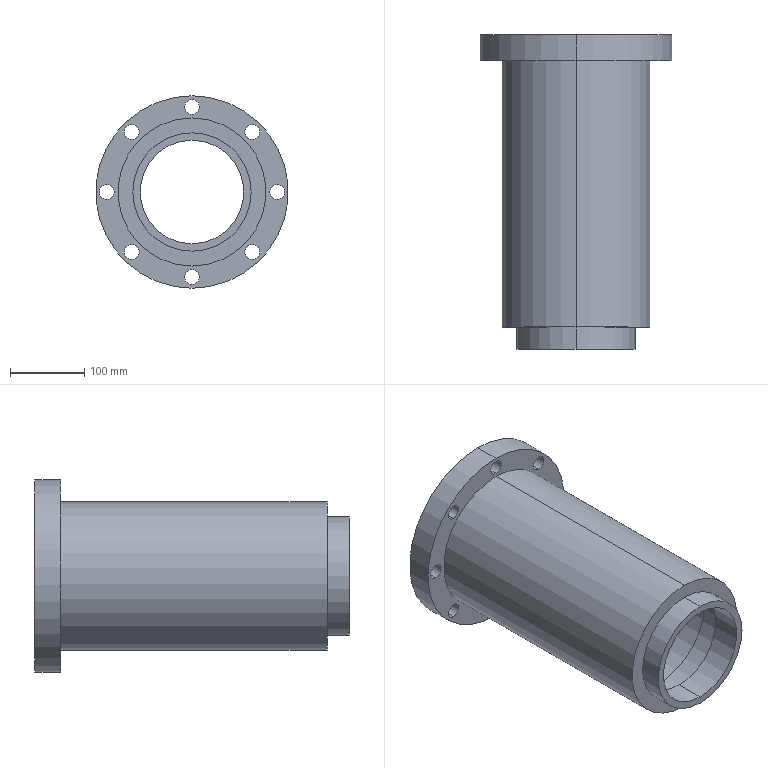Part | SolidWorks | features Cut 3, ICE 2, CirPattern 1, Extrusion 1, Shell 1 | 2 solids | 37 faces | box 260 x 425 x 260 mm | volume 2163536 mm3 | cylinder 30 | plane 7 | commonest cylinder face diameters 20 x16 200 x4 140 x2 160 x2 180 x2 190 x2
STEP:
#1=CARTESIAN_POINT('',(0.,51.,95.));
#2=VERTEX_POINT('',#1);
#3=CARTESIAN_POINT('',(0.,51.,-95.));
#4=VERTEX_POINT('',#3);
#5=CARTESIAN_POINT('',(0.,51.,0.));
#6=DIRECTION('',(0.,-1.,0.));
#7=DIRECTION('',(0.,0.,1.));
#8=AXIS2_PLACEMENT_3D('',#5,#6,#7);
#9=CIRCLE('',#8,95.);
#10=EDGE_CURVE('',#2,#4,#9,.T.);
#11=ORIENTED_EDGE('',*,*,#10,.T.);
#12=CARTESIAN_POINT('',(0.,360.,-95.));
#13=VERTEX_POINT('',#12);
#14=CARTESIAN_POINT('',(0.,-217.701,-95.));
#15=DIRECTION('',(0.,1.,0.));
#16=VECTOR('',#15,1000.);
#17=LINE('',#14,#16);
#18=EDGE_CURVE('',#4,#13,#17,.T.);
#19=ORIENTED_EDGE('',*,*,#18,.T.);
#20=CARTESIAN_POINT('',(0.,360.,95.));
#21=VERTEX_POINT('',#20);
#22=CARTESIAN_POINT('',(0.,360.,0.));
#23=DIRECTION('',(0.,1.,0.));
#24=DIRECTION('',(0.,0.,1.));
#25=AXIS2_PLACEMENT_3D('',#22,#23,#24);
#26=CIRCLE('',#25,95.);
#27=EDGE_CURVE('',#13,#21,#26,.T.);
#28=ORIENTED_EDGE('',*,*,#27,.T.);
#29=CARTESIAN_POINT('',(0.,-217.701,95.));
#30=DIRECTION('',(0.,1.,0.));
#31=VECTOR('',#30,1000.);
#32=LINE('',#29,#31);
#33=EDGE_CURVE('',#2,#21,#32,.T.);
#34=ORIENTED_EDGE('',*,*,#33,.F.);
#35=EDGE_LOOP('',(#11,#19,#28,#34));
#36=FACE_OUTER_BOUND('',#35,.T.);
#37=CARTESIAN_POINT('',(0.,-217.701,0.));
#38=DIRECTION('',(0.,1.,0.));
#39=DIRECTION('',(0.,0.,1.));
#40=AXIS2_PLACEMENT_3D('',#37,#38,#39);
#41=CYLINDRICAL_SURFACE('',#40,95.);
#42=ADVANCED_FACE('',(#36),#41,.F.);
#43=CARTESIAN_POINT('',(0.,-30.,-80.));
#44=VERTEX_POINT('',#43);
#45=CARTESIAN_POINT('',(0.,-30.,80.));
#46=VERTEX_POINT('',#45);
#47=CARTESIAN_POINT('',(0.,-30.,0.));
#48=DIRECTION('',(0.,-1.,0.));
#49=DIRECTION('',(0.,0.,-1.));
#50=AXIS2_PLACEMENT_3D('',#47,#48,#49);
#51=CIRCLE('',#50,80.);
#52=EDGE_CURVE('',#44,#46,#51,.T.);
#53=ORIENTED_EDGE('',*,*,#52,.F.);
#54=CARTESIAN_POINT('',(0.,0.,-80.));
#55=VERTEX_POINT('',#54);
#56=CARTESIAN_POINT('',(0.,-30.,-80.));
#57=DIRECTION('',(0.,1.,0.));
#58=VECTOR('',#57,1000.);
#59=LINE('',#56,#58);
#60=EDGE_CURVE('',#44,#55,#59,.T.);
#61=ORIENTED_EDGE('',*,*,#60,.T.);
#62=CARTESIAN_POINT('',(0.,0.,80.));
#63=VERTEX_POINT('',#62);
#64=CARTESIAN_POINT('',(0.,0.,0.));
#65=DIRECTION('',(0.,-1.,0.));
#66=DIRECTION('',(0.,0.,1.));
#67=AXIS2_PLACEMENT_3D('',#64,#65,#66);
#68=CIRCLE('',#67,80.);
#69=EDGE_CURVE('',#55,#63,#68,.T.);
#70=ORIENTED_EDGE('',*,*,#69,.T.);
#71=CARTESIAN_POINT('',(0.,-30.,80.));
#72=DIRECTION('',(0.,1.,0.));
#73=VECTOR('',#72,1000.);
#74=LINE('',#71,#73);
#75=EDGE_CURVE('',#46,#63,#74,.T.);
#76=ORIENTED_EDGE('',*,*,#75,.F.);
#77=EDGE_LOOP('',(#53,#61,#70,#76));
#78=FACE_OUTER_BOUND('',#77,.T.);
#79=CARTESIAN_POINT('',(0.,-30.,0.));
#80=DIRECTION('',(0.,1.,0.));
#81=DIRECTION('',(0.,0.,1.));
#82=AXIS2_PLACEMENT_3D('',#79,#80,#81);
#83=CYLINDRICAL_SURFACE('',#82,80.);
#84=ADVANCED_FACE('',(#78),#83,.T.);
#85=CARTESIAN_POINT('',(0.,-30.,70.));
#86=VERTEX_POINT('',#85);
#87=CARTESIAN_POINT('',(0.,-30.,-70.));
#88=VERTEX_POINT('',#87);
#89=CARTESIAN_POINT('',(0.,-30.,0.));
#90=DIRECTION('',(0.,-1.,0.));
#91=DIRECTION('',(0.,0.,-1.));
#92=AXIS2_PLACEMENT_3D('',#89,#90,#91);
#93=CIRCLE('',#92,70.);
#94=EDGE_CURVE('',#86,#88,#93,.T.);
#95=ORIENTED_EDGE('',*,*,#94,.T.);
#96=CARTESIAN_POINT('',(0.,10.,-70.));
#97=VERTEX_POINT('',#96);
#98=CARTESIAN_POINT('',(0.,-290.,-70.));
#99=DIRECTION('',(0.,1.,0.));
#100=VECTOR('',#99,1000.);
#101=LINE('',#98,#100);
#102=EDGE_CURVE('',#88,#97,#101,.T.);
#103=ORIENTED_EDGE('',*,*,#102,.T.);
#104=CARTESIAN_POINT('',(0.,10.,70.));
#105=VERTEX_POINT('',#104);
#106=CARTESIAN_POINT('',(0.,10.,0.));
#107=DIRECTION('',(0.,1.,0.));
#108=DIRECTION('',(0.,0.,1.));
#109=AXIS2_PLACEMENT_3D('',#106,#107,#108);
#110=CIRCLE('',#109,70.);
#111=EDGE_CURVE('',#97,#105,#110,.T.);
#112=ORIENTED_EDGE('',*,*,#111,.T.);
#113=CARTESIAN_POINT('',(0.,-290.,70.));
#114=DIRECTION('',(0.,1.,0.));
#115=VECTOR('',#114,1000.);
#116=LINE('',#113,#115);
#117=EDGE_CURVE('',#86,#105,#116,.T.);
#118=ORIENTED_EDGE('',*,*,#117,.F.);
#119=EDGE_LOOP('',(#95,#103,#112,#118));
#120=FACE_OUTER_BOUND('',#119,.T.);
#121=CARTESIAN_POINT('',(0.,-290.,0.));
#122=DIRECTION('',(0.,1.,0.));
#123=DIRECTION('',(0.,0.,1.));
#124=AXIS2_PLACEMENT_3D('',#121,#122,#123);
#125=CYLINDRICAL_SURFACE('',#124,70.);
#126=ADVANCED_FACE('',(#120),#125,.F.);
#127=CARTESIAN_POINT('',(0.,360.,100.));
#128=VERTEX_POINT('',#127);
#129=CARTESIAN_POINT('',(0.,360.,-100.));
#130=VERTEX_POINT('',#129);
#131=CARTESIAN_POINT('',(0.,360.,0.));
#132=DIRECTION('',(0.,1.,0.));
#133=DIRECTION('',(0.,0.,1.));
#134=AXIS2_PLACEMENT_3D('',#131,#132,#133);
#135=CIRCLE('',#134,100.);
#136=EDGE_CURVE('',#128,#130,#135,.T.);
#137=ORIENTED_EDGE('',*,*,#136,.F.);
#138=CARTESIAN_POINT('',(0.,0.,100.));
#139=VERTEX_POINT('',#138);
#140=CARTESIAN_POINT('',(0.,360.,100.));
#141=DIRECTION('',(0.,-1.,0.));
#142=VECTOR('',#141,1000.);
#143=LINE('',#140,#142);
#144=EDGE_CURVE('',#128,#139,#143,.T.);
#145=ORIENTED_EDGE('',*,*,#144,.T.);
#146=CARTESIAN_POINT('',(0.,0.,-100.));
#147=VERTEX_POINT('',#146);
#148=CARTESIAN_POINT('',(0.,0.,0.));
#149=DIRECTION('',(0.,1.,0.));
#150=DIRECTION('',(0.,0.,1.));
#151=AXIS2_PLACEMENT_3D('',#148,#149,#150);
#152=CIRCLE('',#151,100.);
#153=EDGE_CURVE('',#139,#147,#152,.T.);
#154=ORIENTED_EDGE('',*,*,#153,.T.);
#155=CARTESIAN_POINT('',(0.,360.,-100.));
#156=DIRECTION('',(0.,-1.,0.));
#157=VECTOR('',#156,1000.);
#158=LINE('',#155,#157);
#159=EDGE_CURVE('',#130,#147,#158,.T.);
#160=ORIENTED_EDGE('',*,*,#159,.F.);
#161=EDGE_LOOP('',(#137,#145,#154,#160));
#162=FACE_OUTER_BOUND('',#161,.T.);
#163=CARTESIAN_POINT('',(0.,360.,0.));
#164=DIRECTION('',(0.,-1.,0.));
#165=DIRECTION('',(0.,0.,-1.));
#166=AXIS2_PLACEMENT_3D('',#163,#164,#165);
#167=CYLINDRICAL_SURFACE('',#166,100.);
#168=ADVANCED_FACE('',(#162),#167,.T.);
#169=CARTESIAN_POINT('',(0.,51.,90.));
#170=VERTEX_POINT('',#169);
#171=CARTESIAN_POINT('',(0.,51.,-90.));
#172=VERTEX_POINT('',#171);
#173=CARTESIAN_POINT('',(0.,51.,0.));
#174=DIRECTION('',(0.,-1.,0.));
#175=DIRECTION('',(0.,0.,1.));
#176=AXIS2_PLACEMENT_3D('',#173,#174,#175);
#177=CIRCLE('',#176,90.);
#178=EDGE_CURVE('',#170,#172,#177,.T.);
#179=ORIENTED_EDGE('',*,*,#178,.F.);
#180=CARTESIAN_POINT('',(0.,10.,90.));
#181=VERTEX_POINT('',#180);
#182=CARTESIAN_POINT('',(0.,360.,90.));
#183=DIRECTION('',(0.,-1.,0.));
#184=VECTOR('',#183,1000.);
#185=LINE('',#182,#184);
#186=EDGE_CURVE('',#170,#181,#185,.T.);
#187=ORIENTED_EDGE('',*,*,#186,.T.);
#188=CARTESIAN_POINT('',(0.,10.,-90.));
#189=VERTEX_POINT('',#188);
#190=CARTESIAN_POINT('',(0.,10.,0.));
#191=DIRECTION('',(0.,1.,0.));
#192=DIRECTION('',(0.,0.,1.));
#193=AXIS2_PLACEMENT_3D('',#190,#191,#192);
#194=CIRCLE('',#193,90.);
#195=EDGE_CURVE('',#189,#181,#194,.T.);
#196=ORIENTED_EDGE('',*,*,#195,.F.);
#197=CARTESIAN_POINT('',(0.,360.,-90.));
#198=DIRECTION('',(0.,-1.,0.));
#199=VECTOR('',#198,1000.);
#200=LINE('',#197,#199);
#201=EDGE_CURVE('',#172,#189,#200,.T.);
#202=ORIENTED_EDGE('',*,*,#201,.F.);
#203=EDGE_LOOP('',(#179,#187,#196,#202));
#204=FACE_OUTER_BOUND('',#203,.T.);
#205=CARTESIAN_POINT('',(0.,360.,0.));
#206=DIRECTION('',(0.,-1.,0.));
#207=DIRECTION('',(0.,0.,-1.));
#208=AXIS2_PLACEMENT_3D('',#205,#206,#207);
#209=CYLINDRICAL_SURFACE('',#208,90.);
#210=ADVANCED_FACE('',(#204),#209,.F.);
#211=ORIENTED_EDGE('',*,*,#186,.F.);
#212=CARTESIAN_POINT('',(0.,51.,0.));
#213=DIRECTION('',(0.,-1.,0.));
#214=DIRECTION('',(0.,0.,1.));
#215=AXIS2_PLACEMENT_3D('',#212,#213,#214);
#216=CIRCLE('',#215,90.);
#217=EDGE_CURVE('',#172,#170,#216,.T.);
#218=ORIENTED_EDGE('',*,*,#217,.F.);
#219=ORIENTED_EDGE('',*,*,#201,.T.);
#220=CARTESIAN_POINT('',(0.,10.,0.));
#221=DIRECTION('',(0.,1.,0.));
#222=DIRECTION('',(0.,0.,1.));
#223=AXIS2_PLACEMENT_3D('',#220,#221,#222);
#224=CIRCLE('',#223,90.);
#225=EDGE_CURVE('',#181,#189,#224,.T.);
#226=ORIENTED_EDGE('',*,*,#225,.F.);
#227=EDGE_LOOP('',(#211,#218,#219,#226));
#228=FACE_OUTER_BOUND('',#227,.T.);
#229=CARTESIAN_POINT('',(0.,360.,0.));
#230=DIRECTION('',(0.,-1.,0.));
#231=DIRECTION('',(0.,0.,-1.));
#232=AXIS2_PLACEMENT_3D('',#229,#230,#231);
#233=CYLINDRICAL_SURFACE('',#232,90.);
#234=ADVANCED_FACE('',(#228),#233,.F.);
#235=CARTESIAN_POINT('',(0.,0.,0.));
#236=DIRECTION('',(0.,1.,0.));
#237=DIRECTION('',(0.,0.,1.));
#238=AXIS2_PLACEMENT_3D('',#235,#236,#237);
#239=CIRCLE('',#238,100.);
#240=EDGE_CURVE('',#147,#139,#239,.T.);
#241=ORIENTED_EDGE('',*,*,#240,.F.);
#242=ORIENTED_EDGE('',*,*,#153,.F.);
#243=EDGE_LOOP('',(#241,#242));
#244=FACE_OUTER_BOUND('',#243,.T.);
#245=CARTESIAN_POINT('',(0.,0.,0.));
#246=DIRECTION('',(0.,-1.,0.));
#247=DIRECTION('',(0.,0.,1.));
#248=AXIS2_PLACEMENT_3D('',#245,#246,#247);
#249=CIRCLE('',#248,80.);
#250=EDGE_CURVE('',#63,#55,#249,.T.);
#251=ORIENTED_EDGE('',*,*,#250,.F.);
#252=ORIENTED_EDGE('',*,*,#69,.F.);
#253=EDGE_LOOP('',(#251,#252));
#254=FACE_BOUND('',#253,.T.);
#255=CARTESIAN_POINT('',(0.,0.,0.));
#256=DIRECTION('',(0.,1.,0.));
#257=DIRECTION('',(0.,0.,1.));
#258=AXIS2_PLACEMENT_3D('',#255,#256,#257);
#259=PLANE('',#258);
#260=ADVANCED_FACE('',(#244,#254),#259,.F.);
#261=ORIENTED_EDGE('',*,*,#144,.F.);
#262=CARTESIAN_POINT('',(0.,360.,0.));
#263=DIRECTION('',(0.,1.,0.));
#264=DIRECTION('',(0.,0.,1.));
#265=AXIS2_PLACEMENT_3D('',#262,#263,#264);
#266=CIRCLE('',#265,100.);
#267=EDGE_CURVE('',#130,#128,#266,.T.);
#268=ORIENTED_EDGE('',*,*,#267,.F.);
#269=ORIENTED_EDGE('',*,*,#159,.T.);
#270=ORIENTED_EDGE('',*,*,#240,.T.);
#271=EDGE_LOOP('',(#261,#268,#269,#270));
#272=FACE_OUTER_BOUND('',#271,.T.);
#273=CARTESIAN_POINT('',(0.,360.,0.));
#274=DIRECTION('',(0.,-1.,0.));
#275=DIRECTION('',(0.,0.,-1.));
#276=AXIS2_PLACEMENT_3D('',#273,#274,#275);
#277=CYLINDRICAL_SURFACE('',#276,100.);
#278=ADVANCED_FACE('',(#272),#277,.T.);
#279=CARTESIAN_POINT('',(0.,360.,0.));
#280=DIRECTION('',(0.,1.,0.));
#281=DIRECTION('',(0.,0.,1.));
#282=AXIS2_PLACEMENT_3D('',#279,#280,#281);
#283=CIRCLE('',#282,95.);
#284=EDGE_CURVE('',#21,#13,#283,.T.);
#285=ORIENTED_EDGE('',*,*,#284,.F.);
#286=ORIENTED_EDGE('',*,*,#27,.F.);
#287=EDGE_LOOP('',(#285,#286));
#288=FACE_BOUND('',#287,.T.);
#289=ORIENTED_EDGE('',*,*,#267,.T.);
#290=ORIENTED_EDGE('',*,*,#136,.T.);
#291=EDGE_LOOP('',(#289,#290));
#292=FACE_OUTER_BOUND('',#291,.T.);
#293=CARTESIAN_POINT('',(0.,360.,0.));
#294=DIRECTION('',(0.,1.,0.));
#295=DIRECTION('',(0.,0.,1.));
#296=AXIS2_PLACEMENT_3D('',#293,#294,#295);
#297=PLANE('',#296);
#298=ADVANCED_FACE('',(#288,#292),#297,.T.);
#299=CARTESIAN_POINT('',(0.,10.,0.));
#300=DIRECTION('',(0.,1.,0.));
#301=DIRECTION('',(0.,0.,1.));
#302=AXIS2_PLACEMENT_3D('',#299,#300,#301);
#303=CIRCLE('',#302,70.);
#304=EDGE_CURVE('',#105,#97,#303,.T.);
#305=ORIENTED_EDGE('',*,*,#304,.F.);
#306=ORIENTED_EDGE('',*,*,#111,.F.);
#307=EDGE_LOOP('',(#305,#306));
#308=FACE_BOUND('',#307,.T.);
#309=ORIENTED_EDGE('',*,*,#195,.T.);
#310=ORIENTED_EDGE('',*,*,#225,.T.);
#311=EDGE_LOOP('',(#309,#310));
#312=FACE_OUTER_BOUND('',#311,.T.);
#313=CARTESIAN_POINT('',(0.,10.,0.));
#314=DIRECTION('',(0.,1.,0.));
#315=DIRECTION('',(0.,0.,1.));
#316=AXIS2_PLACEMENT_3D('',#313,#314,#315);
#317=PLANE('',#316);
#318=ADVANCED_FACE('',(#308,#312),#317,.T.);
#319=ORIENTED_EDGE('',*,*,#102,.F.);
#320=CARTESIAN_POINT('',(0.,-30.,0.));
#321=DIRECTION('',(0.,-1.,0.));
#322=DIRECTION('',(0.,0.,-1.));
#323=AXIS2_PLACEMENT_3D('',#320,#321,#322);
#324=CIRCLE('',#323,70.);
#325=EDGE_CURVE('',#88,#86,#324,.T.);
#326=ORIENTED_EDGE('',*,*,#325,.T.);
#327=ORIENTED_EDGE('',*,*,#117,.T.);
#328=ORIENTED_EDGE('',*,*,#304,.T.);
#329=EDGE_LOOP('',(#319,#326,#327,#328));
#330=FACE_OUTER_BOUND('',#329,.T.);
#331=CARTESIAN_POINT('',(0.,-290.,0.));
#332=DIRECTION('',(0.,1.,0.));
#333=DIRECTION('',(0.,0.,1.));
#334=AXIS2_PLACEMENT_3D('',#331,#332,#333);
#335=CYLINDRICAL_SURFACE('',#334,70.);
#336=ADVANCED_FACE('',(#330),#335,.F.);
#337=CARTESIAN_POINT('',(0.,-30.,0.));
#338=DIRECTION('',(0.,-1.,0.));
#339=DIRECTION('',(0.,0.,-1.));
#340=AXIS2_PLACEMENT_3D('',#337,#338,#339);
#341=CIRCLE('',#340,80.);
#342=EDGE_CURVE('',#46,#44,#341,.T.);
#343=ORIENTED_EDGE('',*,*,#342,.T.);
#344=ORIENTED_EDGE('',*,*,#52,.T.);
#345=EDGE_LOOP('',(#343,#344));
#346=FACE_OUTER_BOUND('',#345,.T.);
#347=ORIENTED_EDGE('',*,*,#94,.F.);
#348=ORIENTED_EDGE('',*,*,#325,.F.);
#349=EDGE_LOOP('',(#347,#348));
#350=FACE_BOUND('',#349,.T.);
#351=CARTESIAN_POINT('',(0.,-30.,0.));
#352=DIRECTION('',(0.,-1.,0.));
#353=DIRECTION('',(0.,0.,-1.));
#354=AXIS2_PLACEMENT_3D('',#351,#352,#353);
#355=PLANE('',#354);
#356=ADVANCED_FACE('',(#346,#350),#355,.T.);
#357=ORIENTED_EDGE('',*,*,#60,.F.);
#358=ORIENTED_EDGE('',*,*,#342,.F.);
#359=ORIENTED_EDGE('',*,*,#75,.T.);
#360=ORIENTED_EDGE('',*,*,#250,.T.);
#361=EDGE_LOOP('',(#357,#358,#359,#360));
#362=FACE_OUTER_BOUND('',#361,.T.);
#363=CARTESIAN_POINT('',(0.,-30.,0.));
#364=DIRECTION('',(0.,1.,0.));
#365=DIRECTION('',(0.,0.,1.));
#366=AXIS2_PLACEMENT_3D('',#363,#364,#365);
#367=CYLINDRICAL_SURFACE('',#366,80.);
#368=ADVANCED_FACE('',(#362),#367,.T.);
#369=ORIENTED_EDGE('',*,*,#18,.F.);
#370=CARTESIAN_POINT('',(0.,51.,0.));
#371=DIRECTION('',(0.,-1.,0.));
#372=DIRECTION('',(0.,0.,1.));
#373=AXIS2_PLACEMENT_3D('',#370,#371,#372);
#374=CIRCLE('',#373,95.);
#375=EDGE_CURVE('',#4,#2,#374,.T.);
#376=ORIENTED_EDGE('',*,*,#375,.T.);
#377=ORIENTED_EDGE('',*,*,#33,.T.);
#378=ORIENTED_EDGE('',*,*,#284,.T.);
#379=EDGE_LOOP('',(#369,#376,#377,#378));
#380=FACE_OUTER_BOUND('',#379,.T.);
#381=CARTESIAN_POINT('',(0.,-217.701,0.));
#382=DIRECTION('',(0.,1.,0.));
#383=DIRECTION('',(0.,0.,1.));
#384=AXIS2_PLACEMENT_3D('',#381,#382,#383);
#385=CYLINDRICAL_SURFACE('',#384,95.);
#386=ADVANCED_FACE('',(#380),#385,.F.);
#387=ORIENTED_EDGE('',*,*,#10,.F.);
#388=ORIENTED_EDGE('',*,*,#375,.F.);
#389=EDGE_LOOP('',(#387,#388));
#390=FACE_OUTER_BOUND('',#389,.T.);
#391=ORIENTED_EDGE('',*,*,#217,.T.);
#392=ORIENTED_EDGE('',*,*,#178,.T.);
#393=EDGE_LOOP('',(#391,#392));
#394=FACE_BOUND('',#393,.T.);
#395=CARTESIAN_POINT('',(0.,51.,0.));
#396=DIRECTION('',(0.,1.,0.));
#397=DIRECTION('',(-0.9024,0.,-0.4308));
#398=AXIS2_PLACEMENT_3D('',#395,#396,#397);
#399=PLANE('',#398);
#400=ADVANCED_FACE('',(#390,#394),#399,.T.);
#401=CLOSED_SHELL('',(#42,#84,#126,#168,#210,#234,#260,#278,#298,#318,#336,#356,#368,#386,#400));
#402=MANIFOLD_SOLID_BREP('',#401);
#403=CARTESIAN_POINT('',(0.,360.,105.));
#404=VERTEX_POINT('',#403);
#405=CARTESIAN_POINT('',(0.,360.,125.));
#406=VERTEX_POINT('',#405);
#407=CARTESIAN_POINT('',(0.,360.,115.));
#408=DIRECTION('',(0.,1.,0.));
#409=DIRECTION('',(1.,0.,0.));
#410=AXIS2_PLACEMENT_3D('',#407,#408,#409);
#411=CIRCLE('',#410,10.);
#412=EDGE_CURVE('',#404,#406,#411,.T.);
#413=ORIENTED_EDGE('',*,*,#412,.F.);
#414=CARTESIAN_POINT('',(0.,395.,105.));
#415=VERTEX_POINT('',#414);
#416=CARTESIAN_POINT('',(0.,360.,105.));
#417=DIRECTION('',(0.,1.,0.));
#418=VECTOR('',#417,1000.);
#419=LINE('',#416,#418);
#420=EDGE_CURVE('',#404,#415,#419,.T.);
#421=ORIENTED_EDGE('',*,*,#420,.T.);
#422=CARTESIAN_POINT('',(0.,395.,125.));
#423=VERTEX_POINT('',#422);
#424=CARTESIAN_POINT('',(0.,395.,115.));
#425=DIRECTION('',(0.,1.,0.));
#426=DIRECTION('',(0.,0.,1.));
#427=AXIS2_PLACEMENT_3D('',#424,#425,#426);
#428=CIRCLE('',#427,10.);
#429=EDGE_CURVE('',#415,#423,#428,.T.);
#430=ORIENTED_EDGE('',*,*,#429,.T.);
#431=CARTESIAN_POINT('',(0.,360.,125.));
#432=DIRECTION('',(0.,1.,0.));
#433=VECTOR('',#432,1000.);
#434=LINE('',#431,#433);
#435=EDGE_CURVE('',#406,#423,#434,.T.);
#436=ORIENTED_EDGE('',*,*,#435,.F.);
#437=EDGE_LOOP('',(#413,#421,#430,#436));
#438=FACE_OUTER_BOUND('',#437,.T.);
#439=CARTESIAN_POINT('',(0.,360.,115.));
#440=DIRECTION('',(0.,1.,0.));
#441=DIRECTION('',(0.,0.,1.));
#442=AXIS2_PLACEMENT_3D('',#439,#440,#441);
#443=CYLINDRICAL_SURFACE('',#442,10.);
#444=ADVANCED_FACE('',(#438),#443,.F.);
#445=CARTESIAN_POINT('',(81.317,360.,71.317));
#446=VERTEX_POINT('',#445);
#447=CARTESIAN_POINT('',(81.317,360.,91.317));
#448=VERTEX_POINT('',#447);
#449=CARTESIAN_POINT('',(81.317,360.,81.317));
#450=DIRECTION('',(0.,1.,0.));
#451=DIRECTION('',(0.7071,0.,-0.7071));
#452=AXIS2_PLACEMENT_3D('',#449,#450,#451);
#453=CIRCLE('',#452,10.);
#454=EDGE_CURVE('',#446,#448,#453,.T.);
#455=ORIENTED_EDGE('',*,*,#454,.F.);
#456=CARTESIAN_POINT('',(81.317,395.,71.317));
#457=VERTEX_POINT('',#456);
#458=CARTESIAN_POINT('',(81.317,360.,71.317));
#459=DIRECTION('',(0.,1.,0.));
#460=VECTOR('',#459,1000.);
#461=LINE('',#458,#460);
#462=EDGE_CURVE('',#446,#457,#461,.T.);
#463=ORIENTED_EDGE('',*,*,#462,.T.);
#464=CARTESIAN_POINT('',(81.317,395.,91.317));
#465=VERTEX_POINT('',#464);
#466=CARTESIAN_POINT('',(81.317,395.,81.317));
#467=DIRECTION('',(0.,1.,0.));
#468=DIRECTION('',(0.,0.,1.));
#469=AXIS2_PLACEMENT_3D('',#466,#467,#468);
#470=CIRCLE('',#469,10.);
#471=EDGE_CURVE('',#457,#465,#470,.T.);
#472=ORIENTED_EDGE('',*,*,#471,.T.);
#473=CARTESIAN_POINT('',(81.317,360.,91.317));
#474=DIRECTION('',(0.,1.,0.));
#475=VECTOR('',#474,1000.);
#476=LINE('',#473,#475);
#477=EDGE_CURVE('',#448,#465,#476,.T.);
#478=ORIENTED_EDGE('',*,*,#477,.F.);
#479=EDGE_LOOP('',(#455,#463,#472,#478));
#480=FACE_OUTER_BOUND('',#479,.T.);
#481=CARTESIAN_POINT('',(81.317,360.,81.317));
#482=DIRECTION('',(0.,1.,0.));
#483=DIRECTION('',(0.,0.,1.));
#484=AXIS2_PLACEMENT_3D('',#481,#482,#483);
#485=CYLINDRICAL_SURFACE('',#484,10.);
#486=ADVANCED_FACE('',(#480),#485,.F.);
#487=CARTESIAN_POINT('',(115.,360.,-10.));
#488=VERTEX_POINT('',#487);
#489=CARTESIAN_POINT('',(115.,360.,10.));
#490=VERTEX_POINT('',#489);
#491=CARTESIAN_POINT('',(115.,360.,0.));
#492=DIRECTION('',(0.,1.,0.));
#493=DIRECTION('',(0.,0.,-1.));
#494=AXIS2_PLACEMENT_3D('',#491,#492,#493);
#495=CIRCLE('',#494,10.);
#496=EDGE_CURVE('',#488,#490,#495,.T.);
#497=ORIENTED_EDGE('',*,*,#496,.F.);
#498=CARTESIAN_POINT('',(115.,395.,-10.));
#499=VERTEX_POINT('',#498);
#500=CARTESIAN_POINT('',(115.,360.,-10.));
#501=DIRECTION('',(0.,1.,0.));
#502=VECTOR('',#501,1000.);
#503=LINE('',#500,#502);
#504=EDGE_CURVE('',#488,#499,#503,.T.);
#505=ORIENTED_EDGE('',*,*,#504,.T.);
#506=CARTESIAN_POINT('',(115.,395.,10.));
#507=VERTEX_POINT('',#506);
#508=CARTESIAN_POINT('',(115.,395.,0.));
#509=DIRECTION('',(0.,1.,0.));
#510=DIRECTION('',(0.,0.,1.));
#511=AXIS2_PLACEMENT_3D('',#508,#509,#510);
#512=CIRCLE('',#511,10.);
#513=EDGE_CURVE('',#499,#507,#512,.T.);
#514=ORIENTED_EDGE('',*,*,#513,.T.);
#515=CARTESIAN_POINT('',(115.,360.,10.));
#516=DIRECTION('',(0.,1.,0.));
#517=VECTOR('',#516,1000.);
#518=LINE('',#515,#517);
#519=EDGE_CURVE('',#490,#507,#518,.T.);
#520=ORIENTED_EDGE('',*,*,#519,.F.);
#521=EDGE_LOOP('',(#497,#505,#514,#520));
#522=FACE_OUTER_BOUND('',#521,.T.);
#523=CARTESIAN_POINT('',(115.,360.,0.));
#524=DIRECTION('',(0.,1.,0.));
#525=DIRECTION('',(0.,0.,1.));
#526=AXIS2_PLACEMENT_3D('',#523,#524,#525);
#527=CYLINDRICAL_SURFACE('',#526,10.);
#528=ADVANCED_FACE('',(#522),#527,.F.);
#529=CARTESIAN_POINT('',(81.317,360.,-91.317));
#530=VERTEX_POINT('',#529);
#531=CARTESIAN_POINT('',(81.317,360.,-71.317));
#532=VERTEX_POINT('',#531);
#533=CARTESIAN_POINT('',(81.317,360.,-81.317));
#534=DIRECTION('',(0.,1.,0.));
#535=DIRECTION('',(-0.7071,0.,-0.7071));
#536=AXIS2_PLACEMENT_3D('',#533,#534,#535);
#537=CIRCLE('',#536,10.);
#538=EDGE_CURVE('',#530,#532,#537,.T.);
#539=ORIENTED_EDGE('',*,*,#538,.F.);
#540=CARTESIAN_POINT('',(81.317,395.,-91.317));
#541=VERTEX_POINT('',#540);
#542=CARTESIAN_POINT('',(81.317,360.,-91.317));
#543=DIRECTION('',(0.,1.,0.));
#544=VECTOR('',#543,1000.);
#545=LINE('',#542,#544);
#546=EDGE_CURVE('',#530,#541,#545,.T.);
#547=ORIENTED_EDGE('',*,*,#546,.T.);
#548=CARTESIAN_POINT('',(81.317,395.,-71.317));
#549=VERTEX_POINT('',#548);
#550=CARTESIAN_POINT('',(81.317,395.,-81.317));
#551=DIRECTION('',(0.,1.,0.));
#552=DIRECTION('',(0.,0.,1.));
#553=AXIS2_PLACEMENT_3D('',#550,#551,#552);
#554=CIRCLE('',#553,10.);
#555=EDGE_CURVE('',#541,#549,#554,.T.);
#556=ORIENTED_EDGE('',*,*,#555,.T.);
#557=CARTESIAN_POINT('',(81.317,360.,-71.317));
#558=DIRECTION('',(0.,1.,0.));
#559=VECTOR('',#558,1000.);
#560=LINE('',#557,#559);
#561=EDGE_CURVE('',#532,#549,#560,.T.);
#562=ORIENTED_EDGE('',*,*,#561,.F.);
#563=EDGE_LOOP('',(#539,#547,#556,#562));
#564=FACE_OUTER_BOUND('',#563,.T.);
#565=CARTESIAN_POINT('',(81.317,360.,-81.317));
#566=DIRECTION('',(0.,1.,0.));
#567=DIRECTION('',(0.,0.,1.));
#568=AXIS2_PLACEMENT_3D('',#565,#566,#567);
#569=CYLINDRICAL_SURFACE('',#568,10.);
#570=ADVANCED_FACE('',(#564),#569,.F.);
#571=CARTESIAN_POINT('',(0.,360.,-125.));
#572=VERTEX_POINT('',#571);
#573=CARTESIAN_POINT('',(0.,360.,-105.));
#574=VERTEX_POINT('',#573);
#575=CARTESIAN_POINT('',(0.,360.,-115.));
#576=DIRECTION('',(0.,1.,0.));
#577=DIRECTION('',(-1.,0.,0.));
#578=AXIS2_PLACEMENT_3D('',#575,#576,#577);
#579=CIRCLE('',#578,10.);
#580=EDGE_CURVE('',#572,#574,#579,.T.);
#581=ORIENTED_EDGE('',*,*,#580,.F.);
#582=CARTESIAN_POINT('',(0.,395.,-125.));
#583=VERTEX_POINT('',#582);
#584=CARTESIAN_POINT('',(0.,360.,-125.));
#585=DIRECTION('',(0.,1.,0.));
#586=VECTOR('',#585,1000.);
#587=LINE('',#584,#586);
#588=EDGE_CURVE('',#572,#583,#587,.T.);
#589=ORIENTED_EDGE('',*,*,#588,.T.);
#590=CARTESIAN_POINT('',(0.,395.,-105.));
#591=VERTEX_POINT('',#590);
#592=CARTESIAN_POINT('',(0.,395.,-115.));
#593=DIRECTION('',(0.,1.,0.));
#594=DIRECTION('',(0.,0.,1.));
#595=AXIS2_PLACEMENT_3D('',#592,#593,#594);
#596=CIRCLE('',#595,10.);
#597=EDGE_CURVE('',#583,#591,#596,.T.);
#598=ORIENTED_EDGE('',*,*,#597,.T.);
#599=CARTESIAN_POINT('',(0.,360.,-105.));
#600=DIRECTION('',(0.,1.,0.));
#601=VECTOR('',#600,1000.);
#602=LINE('',#599,#601);
#603=EDGE_CURVE('',#574,#591,#602,.T.);
#604=ORIENTED_EDGE('',*,*,#603,.F.);
#605=EDGE_LOOP('',(#581,#589,#598,#604));
#606=FACE_OUTER_BOUND('',#605,.T.);
#607=CARTESIAN_POINT('',(0.,360.,-115.));
#608=DIRECTION('',(0.,1.,0.));
#609=DIRECTION('',(0.,0.,1.));
#610=AXIS2_PLACEMENT_3D('',#607,#608,#609);
#611=CYLINDRICAL_SURFACE('',#610,10.);
#612=ADVANCED_FACE('',(#606),#611,.F.);
#613=CARTESIAN_POINT('',(-81.317,360.,-91.317));
#614=VERTEX_POINT('',#613);
#615=CARTESIAN_POINT('',(-81.317,360.,-71.317));
#616=VERTEX_POINT('',#615);
#617=CARTESIAN_POINT('',(-81.317,360.,-81.317));
#618=DIRECTION('',(0.,1.,0.));
#619=DIRECTION('',(-0.7071,0.,0.7071));
#620=AXIS2_PLACEMENT_3D('',#617,#618,#619);
#621=CIRCLE('',#620,10.);
#622=EDGE_CURVE('',#614,#616,#621,.T.);
#623=ORIENTED_EDGE('',*,*,#622,.F.);
#624=CARTESIAN_POINT('',(-81.317,395.,-91.317));
#625=VERTEX_POINT('',#624);
#626=CARTESIAN_POINT('',(-81.317,360.,-91.317));
#627=DIRECTION('',(0.,1.,0.));
#628=VECTOR('',#627,1000.);
#629=LINE('',#626,#628);
#630=EDGE_CURVE('',#614,#625,#629,.T.);
#631=ORIENTED_EDGE('',*,*,#630,.T.);
#632=CARTESIAN_POINT('',(-81.317,395.,-71.317));
#633=VERTEX_POINT('',#632);
#634=CARTESIAN_POINT('',(-81.317,395.,-81.317));
#635=DIRECTION('',(0.,1.,0.));
#636=DIRECTION('',(0.,0.,1.));
#637=AXIS2_PLACEMENT_3D('',#634,#635,#636);
#638=CIRCLE('',#637,10.);
#639=EDGE_CURVE('',#625,#633,#638,.T.);
#640=ORIENTED_EDGE('',*,*,#639,.T.);
#641=CARTESIAN_POINT('',(-81.317,360.,-71.317));
#642=DIRECTION('',(0.,1.,0.));
#643=VECTOR('',#642,1000.);
#644=LINE('',#641,#643);
#645=EDGE_CURVE('',#616,#633,#644,.T.);
#646=ORIENTED_EDGE('',*,*,#645,.F.);
#647=EDGE_LOOP('',(#623,#631,#640,#646));
#648=FACE_OUTER_BOUND('',#647,.T.);
#649=CARTESIAN_POINT('',(-81.317,360.,-81.317));
#650=DIRECTION('',(0.,1.,0.));
#651=DIRECTION('',(0.,0.,1.));
#652=AXIS2_PLACEMENT_3D('',#649,#650,#651);
#653=CYLINDRICAL_SURFACE('',#652,10.);
#654=ADVANCED_FACE('',(#648),#653,.F.);
#655=CARTESIAN_POINT('',(-81.317,360.,71.317));
#656=VERTEX_POINT('',#655);
#657=CARTESIAN_POINT('',(-81.317,360.,91.317));
#658=VERTEX_POINT('',#657);
#659=CARTESIAN_POINT('',(-81.317,360.,81.317));
#660=DIRECTION('',(0.,1.,0.));
#661=DIRECTION('',(0.7071,0.,0.7071));
#662=AXIS2_PLACEMENT_3D('',#659,#660,#661);
#663=CIRCLE('',#662,10.);
#664=EDGE_CURVE('',#656,#658,#663,.T.);
#665=ORIENTED_EDGE('',*,*,#664,.F.);
#666=CARTESIAN_POINT('',(-81.317,395.,71.317));
#667=VERTEX_POINT('',#666);
#668=CARTESIAN_POINT('',(-81.317,360.,71.317));
#669=DIRECTION('',(0.,1.,0.));
#670=VECTOR('',#669,1000.);
#671=LINE('',#668,#670);
#672=EDGE_CURVE('',#656,#667,#671,.T.);
#673=ORIENTED_EDGE('',*,*,#672,.T.);
#674=CARTESIAN_POINT('',(-81.317,395.,91.317));
#675=VERTEX_POINT('',#674);
#676=CARTESIAN_POINT('',(-81.317,395.,81.317));
#677=DIRECTION('',(0.,1.,0.));
#678=DIRECTION('',(0.,0.,1.));
#679=AXIS2_PLACEMENT_3D('',#676,#677,#678);
#680=CIRCLE('',#679,10.);
#681=EDGE_CURVE('',#667,#675,#680,.T.);
#682=ORIENTED_EDGE('',*,*,#681,.T.);
#683=CARTESIAN_POINT('',(-81.317,360.,91.317));
#684=DIRECTION('',(0.,1.,0.));
#685=VECTOR('',#684,1000.);
#686=LINE('',#683,#685);
#687=EDGE_CURVE('',#658,#675,#686,.T.);
#688=ORIENTED_EDGE('',*,*,#687,.F.);
#689=EDGE_LOOP('',(#665,#673,#682,#688));
#690=FACE_OUTER_BOUND('',#689,.T.);
#691=CARTESIAN_POINT('',(-81.317,360.,81.317));
#692=DIRECTION('',(0.,1.,0.));
#693=DIRECTION('',(0.,0.,1.));
#694=AXIS2_PLACEMENT_3D('',#691,#692,#693);
#695=CYLINDRICAL_SURFACE('',#694,10.);
#696=ADVANCED_FACE('',(#690),#695,.F.);
#697=CARTESIAN_POINT('',(-115.,360.,-10.));
#698=VERTEX_POINT('',#697);
#699=CARTESIAN_POINT('',(-115.,360.,10.));
#700=VERTEX_POINT('',#699);
#701=CARTESIAN_POINT('',(-115.,360.,0.));
#702=DIRECTION('',(0.,1.,0.));
#703=DIRECTION('',(0.,0.,1.));
#704=AXIS2_PLACEMENT_3D('',#701,#702,#703);
#705=CIRCLE('',#704,10.);
#706=EDGE_CURVE('',#698,#700,#705,.T.);
#707=ORIENTED_EDGE('',*,*,#706,.F.);
#708=CARTESIAN_POINT('',(-115.,395.,-10.));
#709=VERTEX_POINT('',#708);
#710=CARTESIAN_POINT('',(-115.,-30.,-10.));
#711=DIRECTION('',(0.,1.,0.));
#712=VECTOR('',#711,1000.);
#713=LINE('',#710,#712);
#714=EDGE_CURVE('',#698,#709,#713,.T.);
#715=ORIENTED_EDGE('',*,*,#714,.T.);
#716=CARTESIAN_POINT('',(-115.,395.,10.));
#717=VERTEX_POINT('',#716);
#718=CARTESIAN_POINT('',(-115.,395.,0.));
#719=DIRECTION('',(0.,1.,0.));
#720=DIRECTION('',(0.,0.,1.));
#721=AXIS2_PLACEMENT_3D('',#718,#719,#720);
#722=CIRCLE('',#721,10.);
#723=EDGE_CURVE('',#709,#717,#722,.T.);
#724=ORIENTED_EDGE('',*,*,#723,.T.);
#725=CARTESIAN_POINT('',(-115.,-30.,10.));
#726=DIRECTION('',(0.,1.,0.));
#727=VECTOR('',#726,1000.);
#728=LINE('',#725,#727);
#729=EDGE_CURVE('',#700,#717,#728,.T.);
#730=ORIENTED_EDGE('',*,*,#729,.F.);
#731=EDGE_LOOP('',(#707,#715,#724,#730));
#732=FACE_OUTER_BOUND('',#731,.T.);
#733=CARTESIAN_POINT('',(-115.,-30.,0.));
#734=DIRECTION('',(0.,1.,0.));
#735=DIRECTION('',(0.,0.,1.));
#736=AXIS2_PLACEMENT_3D('',#733,#734,#735);
#737=CYLINDRICAL_SURFACE('',#736,10.);
#738=ADVANCED_FACE('',(#732),#737,.F.);
#739=CARTESIAN_POINT('',(0.,395.,-100.));
#740=VERTEX_POINT('',#739);
#741=CARTESIAN_POINT('',(0.,395.,100.));
#742=VERTEX_POINT('',#741);
#743=CARTESIAN_POINT('',(0.,395.,0.));
#744=DIRECTION('',(0.,1.,0.));
#745=DIRECTION('',(0.,0.,1.));
#746=AXIS2_PLACEMENT_3D('',#743,#744,#745);
#747=CIRCLE('',#746,100.);
#748=EDGE_CURVE('',#740,#742,#747,.T.);
#749=ORIENTED_EDGE('',*,*,#748,.T.);
#750=CARTESIAN_POINT('',(0.,360.,100.));
#751=VERTEX_POINT('',#750);
#752=CARTESIAN_POINT('',(0.,395.,100.));
#753=DIRECTION('',(0.,-1.,0.));
#754=VECTOR('',#753,1000.);
#755=LINE('',#752,#754);
#756=EDGE_CURVE('',#742,#751,#755,.T.);
#757=ORIENTED_EDGE('',*,*,#756,.T.);
#758=CARTESIAN_POINT('',(0.,360.,-100.));
#759=VERTEX_POINT('',#758);
#760=CARTESIAN_POINT('',(0.,360.,0.));
#761=DIRECTION('',(0.,1.,0.));
#762=DIRECTION('',(0.,0.,1.));
#763=AXIS2_PLACEMENT_3D('',#760,#761,#762);
#764=CIRCLE('',#763,100.);
#765=EDGE_CURVE('',#759,#751,#764,.T.);
#766=ORIENTED_EDGE('',*,*,#765,.F.);
#767=CARTESIAN_POINT('',(0.,395.,-100.));
#768=DIRECTION('',(0.,-1.,0.));
#769=VECTOR('',#768,1000.);
#770=LINE('',#767,#769);
#771=EDGE_CURVE('',#740,#759,#770,.T.);
#772=ORIENTED_EDGE('',*,*,#771,.F.);
#773=EDGE_LOOP('',(#749,#757,#766,#772));
#774=FACE_OUTER_BOUND('',#773,.T.);
#775=CARTESIAN_POINT('',(0.,395.,0.));
#776=DIRECTION('',(0.,-1.,0.));
#777=DIRECTION('',(0.,0.,-1.));
#778=AXIS2_PLACEMENT_3D('',#775,#776,#777);
#779=CYLINDRICAL_SURFACE('',#778,100.);
#780=ADVANCED_FACE('',(#774),#779,.F.);
#781=CARTESIAN_POINT('',(0.,395.,130.));
#782=VERTEX_POINT('',#781);
#783=CARTESIAN_POINT('',(0.,395.,-130.));
#784=VERTEX_POINT('',#783);
#785=CARTESIAN_POINT('',(0.,395.,0.));
#786=DIRECTION('',(0.,1.,0.));
#787=DIRECTION('',(0.,0.,1.));
#788=AXIS2_PLACEMENT_3D('',#785,#786,#787);
#789=CIRCLE('',#788,130.);
#790=EDGE_CURVE('',#782,#784,#789,.T.);
#791=ORIENTED_EDGE('',*,*,#790,.F.);
#792=CARTESIAN_POINT('',(0.,360.,130.));
#793=VERTEX_POINT('',#792);
#794=CARTESIAN_POINT('',(0.,395.,130.));
#795=DIRECTION('',(0.,-1.,0.));
#796=VECTOR('',#795,1000.);
#797=LINE('',#794,#796);
#798=EDGE_CURVE('',#782,#793,#797,.T.);
#799=ORIENTED_EDGE('',*,*,#798,.T.);
#800=CARTESIAN_POINT('',(0.,360.,-130.));
#801=VERTEX_POINT('',#800);
#802=CARTESIAN_POINT('',(0.,360.,0.));
#803=DIRECTION('',(0.,1.,0.));
#804=DIRECTION('',(0.,0.,1.));
#805=AXIS2_PLACEMENT_3D('',#802,#803,#804);
#806=CIRCLE('',#805,130.);
#807=EDGE_CURVE('',#793,#801,#806,.T.);
#808=ORIENTED_EDGE('',*,*,#807,.T.);
#809=CARTESIAN_POINT('',(0.,395.,-130.));
#810=DIRECTION('',(0.,-1.,0.));
#811=VECTOR('',#810,1000.);
#812=LINE('',#809,#811);
#813=EDGE_CURVE('',#784,#801,#812,.T.);
#814=ORIENTED_EDGE('',*,*,#813,.F.);
#815=EDGE_LOOP('',(#791,#799,#808,#814));
#816=FACE_OUTER_BOUND('',#815,.T.);
#817=CARTESIAN_POINT('',(0.,395.,0.));
#818=DIRECTION('',(0.,-1.,0.));
#819=DIRECTION('',(0.,0.,-1.));
#820=AXIS2_PLACEMENT_3D('',#817,#818,#819);
#821=CYLINDRICAL_SURFACE('',#820,130.);
#822=ADVANCED_FACE('',(#816),#821,.T.);
#823=CARTESIAN_POINT('',(0.,395.,115.));
#824=DIRECTION('',(0.,1.,0.));
#825=DIRECTION('',(0.,0.,1.));
#826=AXIS2_PLACEMENT_3D('',#823,#824,#825);
#827=CIRCLE('',#826,10.);
#828=EDGE_CURVE('',#423,#415,#827,.T.);
#829=ORIENTED_EDGE('',*,*,#828,.F.);
#830=ORIENTED_EDGE('',*,*,#429,.F.);
#831=EDGE_LOOP('',(#829,#830));
#832=FACE_BOUND('',#831,.T.);
#833=CARTESIAN_POINT('',(81.317,395.,81.317));
#834=DIRECTION('',(0.,1.,0.));
#835=DIRECTION('',(0.,0.,1.));
#836=AXIS2_PLACEMENT_3D('',#833,#834,#835);
#837=CIRCLE('',#836,10.);
#838=EDGE_CURVE('',#465,#457,#837,.T.);
#839=ORIENTED_EDGE('',*,*,#838,.F.);
#840=ORIENTED_EDGE('',*,*,#471,.F.);
#841=EDGE_LOOP('',(#839,#840));
#842=FACE_BOUND('',#841,.T.);
#843=CARTESIAN_POINT('',(115.,395.,0.));
#844=DIRECTION('',(0.,1.,0.));
#845=DIRECTION('',(0.,0.,1.));
#846=AXIS2_PLACEMENT_3D('',#843,#844,#845);
#847=CIRCLE('',#846,10.);
#848=EDGE_CURVE('',#507,#499,#847,.T.);
#849=ORIENTED_EDGE('',*,*,#848,.F.);
#850=ORIENTED_EDGE('',*,*,#513,.F.);
#851=EDGE_LOOP('',(#849,#850));
#852=FACE_BOUND('',#851,.T.);
#853=CARTESIAN_POINT('',(81.317,395.,-81.317));
#854=DIRECTION('',(0.,1.,0.));
#855=DIRECTION('',(0.,0.,1.));
#856=AXIS2_PLACEMENT_3D('',#853,#854,#855);
#857=CIRCLE('',#856,10.);
#858=EDGE_CURVE('',#549,#541,#857,.T.);
#859=ORIENTED_EDGE('',*,*,#858,.F.);
#860=ORIENTED_EDGE('',*,*,#555,.F.);
#861=EDGE_LOOP('',(#859,#860));
#862=FACE_BOUND('',#861,.T.);
#863=CARTESIAN_POINT('',(0.,395.,-115.));
#864=DIRECTION('',(0.,1.,0.));
#865=DIRECTION('',(0.,0.,1.));
#866=AXIS2_PLACEMENT_3D('',#863,#864,#865);
#867=CIRCLE('',#866,10.);
#868=EDGE_CURVE('',#591,#583,#867,.T.);
#869=ORIENTED_EDGE('',*,*,#868,.F.);
#870=ORIENTED_EDGE('',*,*,#597,.F.);
#871=EDGE_LOOP('',(#869,#870));
#872=FACE_BOUND('',#871,.T.);
#873=CARTESIAN_POINT('',(-81.317,395.,-81.317));
#874=DIRECTION('',(0.,1.,0.));
#875=DIRECTION('',(0.,0.,1.));
#876=AXIS2_PLACEMENT_3D('',#873,#874,#875);
#877=CIRCLE('',#876,10.);
#878=EDGE_CURVE('',#633,#625,#877,.T.);
#879=ORIENTED_EDGE('',*,*,#878,.F.);
#880=ORIENTED_EDGE('',*,*,#639,.F.);
#881=EDGE_LOOP('',(#879,#880));
#882=FACE_BOUND('',#881,.T.);
#883=CARTESIAN_POINT('',(-81.317,395.,81.317));
#884=DIRECTION('',(0.,1.,0.));
#885=DIRECTION('',(0.,0.,1.));
#886=AXIS2_PLACEMENT_3D('',#883,#884,#885);
#887=CIRCLE('',#886,10.);
#888=EDGE_CURVE('',#675,#667,#887,.T.);
#889=ORIENTED_EDGE('',*,*,#888,.F.);
#890=ORIENTED_EDGE('',*,*,#681,.F.);
#891=EDGE_LOOP('',(#889,#890));
#892=FACE_BOUND('',#891,.T.);
#893=CARTESIAN_POINT('',(-115.,395.,0.));
#894=DIRECTION('',(0.,1.,0.));
#895=DIRECTION('',(0.,0.,1.));
#896=AXIS2_PLACEMENT_3D('',#893,#894,#895);
#897=CIRCLE('',#896,10.);
#898=EDGE_CURVE('',#717,#709,#897,.T.);
#899=ORIENTED_EDGE('',*,*,#898,.F.);
#900=ORIENTED_EDGE('',*,*,#723,.F.);
#901=EDGE_LOOP('',(#899,#900));
#902=FACE_BOUND('',#901,.T.);
#903=CARTESIAN_POINT('',(0.,395.,0.));
#904=DIRECTION('',(0.,1.,0.));
#905=DIRECTION('',(0.,0.,1.));
#906=AXIS2_PLACEMENT_3D('',#903,#904,#905);
#907=CIRCLE('',#906,130.);
#908=EDGE_CURVE('',#784,#782,#907,.T.);
#909=ORIENTED_EDGE('',*,*,#908,.T.);
#910=ORIENTED_EDGE('',*,*,#790,.T.);
#911=EDGE_LOOP('',(#909,#910));
#912=FACE_OUTER_BOUND('',#911,.T.);
#913=ORIENTED_EDGE('',*,*,#748,.F.);
#914=CARTESIAN_POINT('',(0.,395.,0.));
#915=DIRECTION('',(0.,1.,0.));
#916=DIRECTION('',(0.,0.,1.));
#917=AXIS2_PLACEMENT_3D('',#914,#915,#916);
#918=CIRCLE('',#917,100.);
#919=EDGE_CURVE('',#742,#740,#918,.T.);
#920=ORIENTED_EDGE('',*,*,#919,.F.);
#921=EDGE_LOOP('',(#913,#920));
#922=FACE_BOUND('',#921,.T.);
#923=CARTESIAN_POINT('',(0.,395.,0.));
#924=DIRECTION('',(0.,1.,0.));
#925=DIRECTION('',(0.,0.,1.));
#926=AXIS2_PLACEMENT_3D('',#923,#924,#925);
#927=PLANE('',#926);
#928=ADVANCED_FACE('',(#832,#842,#852,#862,#872,#882,#892,#902,#912,#922),#927,.T.);
#929=CARTESIAN_POINT('',(0.,360.,115.));
#930=DIRECTION('',(0.,1.,0.));
#931=DIRECTION('',(1.,0.,0.));
#932=AXIS2_PLACEMENT_3D('',#929,#930,#931);
#933=CIRCLE('',#932,10.);
#934=EDGE_CURVE('',#406,#404,#933,.T.);
#935=ORIENTED_EDGE('',*,*,#934,.T.);
#936=ORIENTED_EDGE('',*,*,#412,.T.);
#937=EDGE_LOOP('',(#935,#936));
#938=FACE_BOUND('',#937,.T.);
#939=CARTESIAN_POINT('',(81.317,360.,81.317));
#940=DIRECTION('',(0.,1.,0.));
#941=DIRECTION('',(0.7071,0.,-0.7071));
#942=AXIS2_PLACEMENT_3D('',#939,#940,#941);
#943=CIRCLE('',#942,10.);
#944=EDGE_CURVE('',#448,#446,#943,.T.);
#945=ORIENTED_EDGE('',*,*,#944,.T.);
#946=ORIENTED_EDGE('',*,*,#454,.T.);
#947=EDGE_LOOP('',(#945,#946));
#948=FACE_BOUND('',#947,.T.);
#949=CARTESIAN_POINT('',(115.,360.,0.));
#950=DIRECTION('',(0.,1.,0.));
#951=DIRECTION('',(0.,0.,-1.));
#952=AXIS2_PLACEMENT_3D('',#949,#950,#951);
#953=CIRCLE('',#952,10.);
#954=EDGE_CURVE('',#490,#488,#953,.T.);
#955=ORIENTED_EDGE('',*,*,#954,.T.);
#956=ORIENTED_EDGE('',*,*,#496,.T.);
#957=EDGE_LOOP('',(#955,#956));
#958=FACE_BOUND('',#957,.T.);
#959=CARTESIAN_POINT('',(81.317,360.,-81.317));
#960=DIRECTION('',(0.,1.,0.));
#961=DIRECTION('',(-0.7071,0.,-0.7071));
#962=AXIS2_PLACEMENT_3D('',#959,#960,#961);
#963=CIRCLE('',#962,10.);
#964=EDGE_CURVE('',#532,#530,#963,.T.);
#965=ORIENTED_EDGE('',*,*,#964,.T.);
#966=ORIENTED_EDGE('',*,*,#538,.T.);
#967=EDGE_LOOP('',(#965,#966));
#968=FACE_BOUND('',#967,.T.);
#969=CARTESIAN_POINT('',(0.,360.,-115.));
#970=DIRECTION('',(0.,1.,0.));
#971=DIRECTION('',(-1.,0.,0.));
#972=AXIS2_PLACEMENT_3D('',#969,#970,#971);
#973=CIRCLE('',#972,10.);
#974=EDGE_CURVE('',#574,#572,#973,.T.);
#975=ORIENTED_EDGE('',*,*,#974,.T.);
#976=ORIENTED_EDGE('',*,*,#580,.T.);
#977=EDGE_LOOP('',(#975,#976));
#978=FACE_BOUND('',#977,.T.);
#979=CARTESIAN_POINT('',(-81.317,360.,-81.317));
#980=DIRECTION('',(0.,1.,0.));
#981=DIRECTION('',(-0.7071,0.,0.7071));
#982=AXIS2_PLACEMENT_3D('',#979,#980,#981);
#983=CIRCLE('',#982,10.);
#984=EDGE_CURVE('',#616,#614,#983,.T.);
#985=ORIENTED_EDGE('',*,*,#984,.T.);
#986=ORIENTED_EDGE('',*,*,#622,.T.);
#987=EDGE_LOOP('',(#985,#986));
#988=FACE_BOUND('',#987,.T.);
#989=CARTESIAN_POINT('',(-81.317,360.,81.317));
#990=DIRECTION('',(0.,1.,0.));
#991=DIRECTION('',(0.7071,0.,0.7071));
#992=AXIS2_PLACEMENT_3D('',#989,#990,#991);
#993=CIRCLE('',#992,10.);
#994=EDGE_CURVE('',#658,#656,#993,.T.);
#995=ORIENTED_EDGE('',*,*,#994,.T.);
#996=ORIENTED_EDGE('',*,*,#664,.T.);
#997=EDGE_LOOP('',(#995,#996));
#998=FACE_BOUND('',#997,.T.);
#999=CARTESIAN_POINT('',(-115.,360.,0.));
#1000=DIRECTION('',(0.,1.,0.));
#1001=DIRECTION('',(0.,0.,1.));
#1002=AXIS2_PLACEMENT_3D('',#999,#1000,#1001);
#1003=CIRCLE('',#1002,10.);
#1004=EDGE_CURVE('',#700,#698,#1003,.T.);
#1005=ORIENTED_EDGE('',*,*,#1004,.T.);
#1006=ORIENTED_EDGE('',*,*,#706,.T.);
#1007=EDGE_LOOP('',(#1005,#1006));
#1008=FACE_BOUND('',#1007,.T.);
#1009=CARTESIAN_POINT('',(0.,360.,0.));
#1010=DIRECTION('',(0.,1.,0.));
#1011=DIRECTION('',(0.,0.,1.));
#1012=AXIS2_PLACEMENT_3D('',#1009,#1010,#1011);
#1013=CIRCLE('',#1012,130.);
#1014=EDGE_CURVE('',#801,#793,#1013,.T.);
#1015=ORIENTED_EDGE('',*,*,#1014,.F.);
#1016=ORIENTED_EDGE('',*,*,#807,.F.);
#1017=EDGE_LOOP('',(#1015,#1016));
#1018=FACE_OUTER_BOUND('',#1017,.T.);
#1019=ORIENTED_EDGE('',*,*,#765,.T.);
#1020=CARTESIAN_POINT('',(0.,360.,0.));
#1021=DIRECTION('',(0.,1.,0.));
#1022=DIRECTION('',(0.,0.,1.));
#1023=AXIS2_PLACEMENT_3D('',#1020,#1021,#1022);
#1024=CIRCLE('',#1023,100.);
#1025=EDGE_CURVE('',#751,#759,#1024,.T.);
#1026=ORIENTED_EDGE('',*,*,#1025,.T.);
#1027=EDGE_LOOP('',(#1019,#1026));
#1028=FACE_BOUND('',#1027,.T.);
#1029=CARTESIAN_POINT('',(0.,360.,0.));
#1030=DIRECTION('',(0.,1.,0.));
#1031=DIRECTION('',(0.,0.,1.));
#1032=AXIS2_PLACEMENT_3D('',#1029,#1030,#1031);
#1033=PLANE('',#1032);
#1034=ADVANCED_FACE('',(#938,#948,#958,#968,#978,#988,#998,#1008,#1018,#1028),#1033,.F.);
#1035=ORIENTED_EDGE('',*,*,#798,.F.);
#1036=ORIENTED_EDGE('',*,*,#908,.F.);
#1037=ORIENTED_EDGE('',*,*,#813,.T.);
#1038=ORIENTED_EDGE('',*,*,#1014,.T.);
#1039=EDGE_LOOP('',(#1035,#1036,#1037,#1038));
#1040=FACE_OUTER_BOUND('',#1039,.T.);
#1041=CARTESIAN_POINT('',(0.,395.,0.));
#1042=DIRECTION('',(0.,-1.,0.));
#1043=DIRECTION('',(0.,0.,-1.));
#1044=AXIS2_PLACEMENT_3D('',#1041,#1042,#1043);
#1045=CYLINDRICAL_SURFACE('',#1044,130.);
#1046=ADVANCED_FACE('',(#1040),#1045,.T.);
#1047=ORIENTED_EDGE('',*,*,#756,.F.);
#1048=ORIENTED_EDGE('',*,*,#919,.T.);
#1049=ORIENTED_EDGE('',*,*,#771,.T.);
#1050=ORIENTED_EDGE('',*,*,#1025,.F.);
#1051=EDGE_LOOP('',(#1047,#1048,#1049,#1050));
#1052=FACE_OUTER_BOUND('',#1051,.T.);
#1053=CARTESIAN_POINT('',(0.,395.,0.));
#1054=DIRECTION('',(0.,-1.,0.));
#1055=DIRECTION('',(0.,0.,-1.));
#1056=AXIS2_PLACEMENT_3D('',#1053,#1054,#1055);
#1057=CYLINDRICAL_SURFACE('',#1056,100.);
#1058=ADVANCED_FACE('',(#1052),#1057,.F.);
#1059=ORIENTED_EDGE('',*,*,#714,.F.);
#1060=ORIENTED_EDGE('',*,*,#1004,.F.);
#1061=ORIENTED_EDGE('',*,*,#729,.T.);
#1062=ORIENTED_EDGE('',*,*,#898,.T.);
#1063=EDGE_LOOP('',(#1059,#1060,#1061,#1062));
#1064=FACE_OUTER_BOUND('',#1063,.T.);
#1065=CARTESIAN_POINT('',(-115.,-30.,0.));
#1066=DIRECTION('',(0.,1.,0.));
#1067=DIRECTION('',(0.,0.,1.));
#1068=AXIS2_PLACEMENT_3D('',#1065,#1066,#1067);
#1069=CYLINDRICAL_SURFACE('',#1068,10.);
#1070=ADVANCED_FACE('',(#1064),#1069,.F.);
#1071=ORIENTED_EDGE('',*,*,#672,.F.);
#1072=ORIENTED_EDGE('',*,*,#994,.F.);
#1073=ORIENTED_EDGE('',*,*,#687,.T.);
#1074=ORIENTED_EDGE('',*,*,#888,.T.);
#1075=EDGE_LOOP('',(#1071,#1072,#1073,#1074));
#1076=FACE_OUTER_BOUND('',#1075,.T.);
#1077=CARTESIAN_POINT('',(-81.317,360.,81.317));
#1078=DIRECTION('',(0.,1.,0.));
#1079=DIRECTION('',(0.,0.,1.));
#1080=AXIS2_PLACEMENT_3D('',#1077,#1078,#1079);
#1081=CYLINDRICAL_SURFACE('',#1080,10.);
#1082=ADVANCED_FACE('',(#1076),#1081,.F.);
#1083=ORIENTED_EDGE('',*,*,#630,.F.);
#1084=ORIENTED_EDGE('',*,*,#984,.F.);
#1085=ORIENTED_EDGE('',*,*,#645,.T.);
#1086=ORIENTED_EDGE('',*,*,#878,.T.);
#1087=EDGE_LOOP('',(#1083,#1084,#1085,#1086));
#1088=FACE_OUTER_BOUND('',#1087,.T.);
#1089=CARTESIAN_POINT('',(-81.317,360.,-81.317));
#1090=DIRECTION('',(0.,1.,0.));
#1091=DIRECTION('',(0.,0.,1.));
#1092=AXIS2_PLACEMENT_3D('',#1089,#1090,#1091);
#1093=CYLINDRICAL_SURFACE('',#1092,10.);
#1094=ADVANCED_FACE('',(#1088),#1093,.F.);
#1095=ORIENTED_EDGE('',*,*,#588,.F.);
#1096=ORIENTED_EDGE('',*,*,#974,.F.);
#1097=ORIENTED_EDGE('',*,*,#603,.T.);
#1098=ORIENTED_EDGE('',*,*,#868,.T.);
#1099=EDGE_LOOP('',(#1095,#1096,#1097,#1098));
#1100=FACE_OUTER_BOUND('',#1099,.T.);
#1101=CARTESIAN_POINT('',(0.,360.,-115.));
#1102=DIRECTION('',(0.,1.,0.));
#1103=DIRECTION('',(0.,0.,1.));
#1104=AXIS2_PLACEMENT_3D('',#1101,#1102,#1103);
#1105=CYLINDRICAL_SURFACE('',#1104,10.);
#1106=ADVANCED_FACE('',(#1100),#1105,.F.);
#1107=ORIENTED_EDGE('',*,*,#546,.F.);
#1108=ORIENTED_EDGE('',*,*,#964,.F.);
#1109=ORIENTED_EDGE('',*,*,#561,.T.);
#1110=ORIENTED_EDGE('',*,*,#858,.T.);
#1111=EDGE_LOOP('',(#1107,#1108,#1109,#1110));
#1112=FACE_OUTER_BOUND('',#1111,.T.);
#1113=CARTESIAN_POINT('',(81.317,360.,-81.317));
#1114=DIRECTION('',(0.,1.,0.));
#1115=DIRECTION('',(0.,0.,1.));
#1116=AXIS2_PLACEMENT_3D('',#1113,#1114,#1115);
#1117=CYLINDRICAL_SURFACE('',#1116,10.);
#1118=ADVANCED_FACE('',(#1112),#1117,.F.);
#1119=ORIENTED_EDGE('',*,*,#504,.F.);
#1120=ORIENTED_EDGE('',*,*,#954,.F.);
#1121=ORIENTED_EDGE('',*,*,#519,.T.);
#1122=ORIENTED_EDGE('',*,*,#848,.T.);
#1123=EDGE_LOOP('',(#1119,#1120,#1121,#1122));
#1124=FACE_OUTER_BOUND('',#1123,.T.);
#1125=CARTESIAN_POINT('',(115.,360.,0.));
#1126=DIRECTION('',(0.,1.,0.));
#1127=DIRECTION('',(0.,0.,1.));
#1128=AXIS2_PLACEMENT_3D('',#1125,#1126,#1127);
#1129=CYLINDRICAL_SURFACE('',#1128,10.);
#1130=ADVANCED_FACE('',(#1124),#1129,.F.);
#1131=ORIENTED_EDGE('',*,*,#462,.F.);
#1132=ORIENTED_EDGE('',*,*,#944,.F.);
#1133=ORIENTED_EDGE('',*,*,#477,.T.);
#1134=ORIENTED_EDGE('',*,*,#838,.T.);
#1135=EDGE_LOOP('',(#1131,#1132,#1133,#1134));
#1136=FACE_OUTER_BOUND('',#1135,.T.);
#1137=CARTESIAN_POINT('',(81.317,360.,81.317));
#1138=DIRECTION('',(0.,1.,0.));
#1139=DIRECTION('',(0.,0.,1.));
#1140=AXIS2_PLACEMENT_3D('',#1137,#1138,#1139);
#1141=CYLINDRICAL_SURFACE('',#1140,10.);
#1142=ADVANCED_FACE('',(#1136),#1141,.F.);
#1143=ORIENTED_EDGE('',*,*,#420,.F.);
#1144=ORIENTED_EDGE('',*,*,#934,.F.);
#1145=ORIENTED_EDGE('',*,*,#435,.T.);
#1146=ORIENTED_EDGE('',*,*,#828,.T.);
#1147=EDGE_LOOP('',(#1143,#1144,#1145,#1146));
#1148=FACE_OUTER_BOUND('',#1147,.T.);
#1149=CARTESIAN_POINT('',(0.,360.,115.));
#1150=DIRECTION('',(0.,1.,0.));
#1151=DIRECTION('',(0.,0.,1.));
#1152=AXIS2_PLACEMENT_3D('',#1149,#1150,#1151);
#1153=CYLINDRICAL_SURFACE('',#1152,10.);
#1154=ADVANCED_FACE('',(#1148),#1153,.F.);
#1155=CLOSED_SHELL('',(#444,#486,#528,#570,#612,#654,#696,#738,#780,#822,#928,#1034,#1046,#1058,#1070,#1082,#1094,#1106,#1118,#1130,#1142,#1154));
#1156=MANIFOLD_SOLID_BREP('',#1155);
#1157=CARTESIAN_POINT('',(0.,0.,0.));
#1158=DIRECTION('',(0.,0.,1.));
#1159=DIRECTION('',(1.,0.,0.));
#1160=AXIS2_PLACEMENT_3D('',#1157,#1158,#1159);
#1161=(LENGTH_UNIT()NAMED_UNIT(*)SI_UNIT(.MILLI.,.METRE.));
#1162=UNCERTAINTY_MEASURE_WITH_UNIT(LENGTH_MEASURE(0.00001),#1161,'','');
#1163=(NAMED_UNIT(*)PLANE_ANGLE_UNIT()SI_UNIT($,.RADIAN.));
#1164=(NAMED_UNIT(*)SI_UNIT($,.STERADIAN.)SOLID_ANGLE_UNIT());
#1165=(GEOMETRIC_REPRESENTATION_CONTEXT(3)GLOBAL_UNCERTAINTY_ASSIGNED_CONTEXT((#1162))GLOBAL_UNIT_ASSIGNED_CONTEXT((#1161,#1163,#1164))REPRESENTATION_CONTEXT('',''));
#1166=ADVANCED_BREP_SHAPE_REPRESENTATION('',(#402,#1156,#1160),#1165);